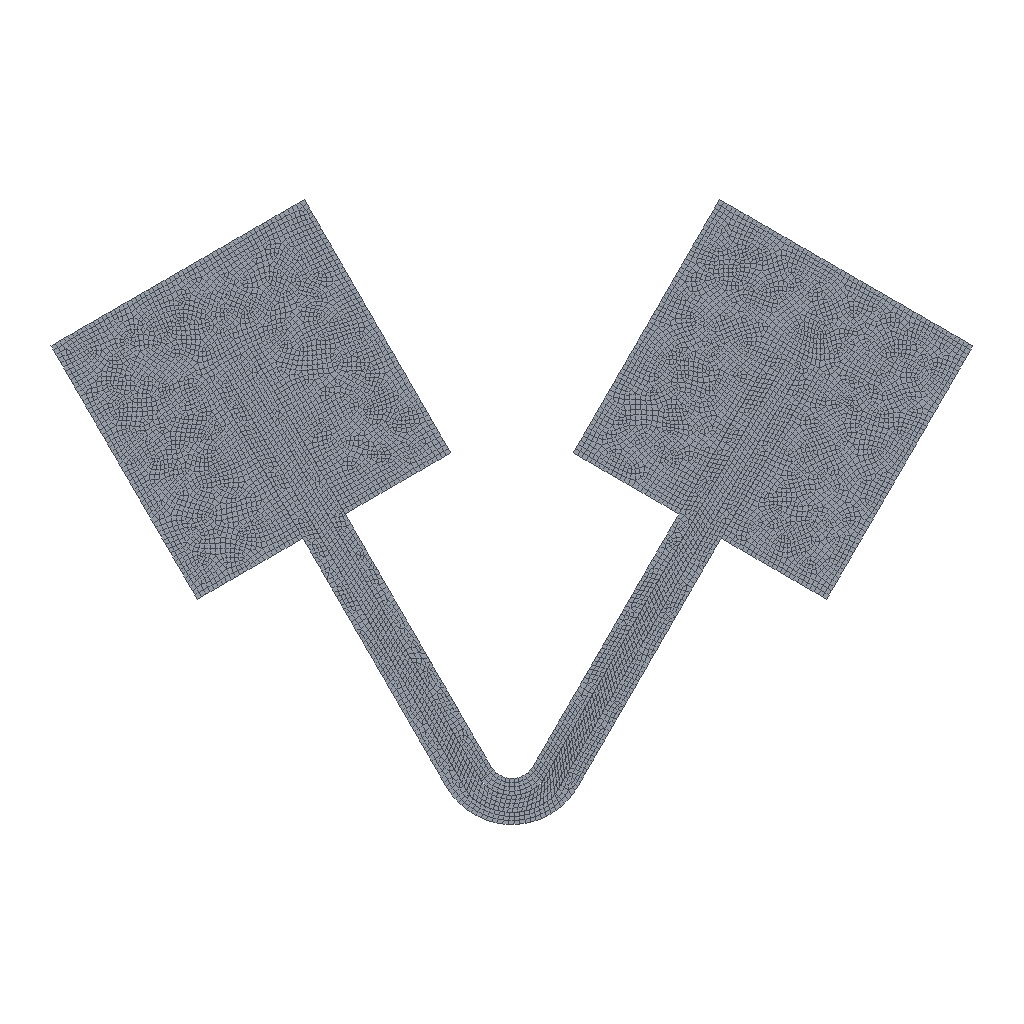Simulation study | abaqus
Set-up summary:
category,name,step,type,value,unit,region
solver,abaqus
solver,version,,,Abaqus/Explicit 3DEXPERIENCE R2017x
units,not stated in the deck,,not stated
analysis,deck,,transient,transient
load_step,Step-1,Step-1,transient,nlgeom=True
contact,interactions,,,general=0 pairs=3 ties=0
load_step,requested,,,1
mesh,nodes,,,11215
mesh,elements,,,10222
element_type,CPS4R,,plane,10222
load,load commands in deck,,count,2
bc,support commands in deck,,count,4
material,BASE,,in results
material,BASE-COPY,,in results
material,FIBER,,in results
check,setup vs results,,match,"per instance, exact: element labels, types and connectivity; labels of the nodes the elements use; coordinates of those nodes at SINGLE_PRECISION in 4 of 4 instance(s)"
Results summary:
result,step,Step-1,completed,increments=1224794 time=0.1/0.1
result,analysis,,,transient
result,last_loadstep,,,1
result,analysis steps,,count,1
result,primary field,,,U
result,reaction total,,FX,-13.271,model units
result,reaction total,,FY,-14.063,model units
result,reaction total,,FZ,0.0,model units